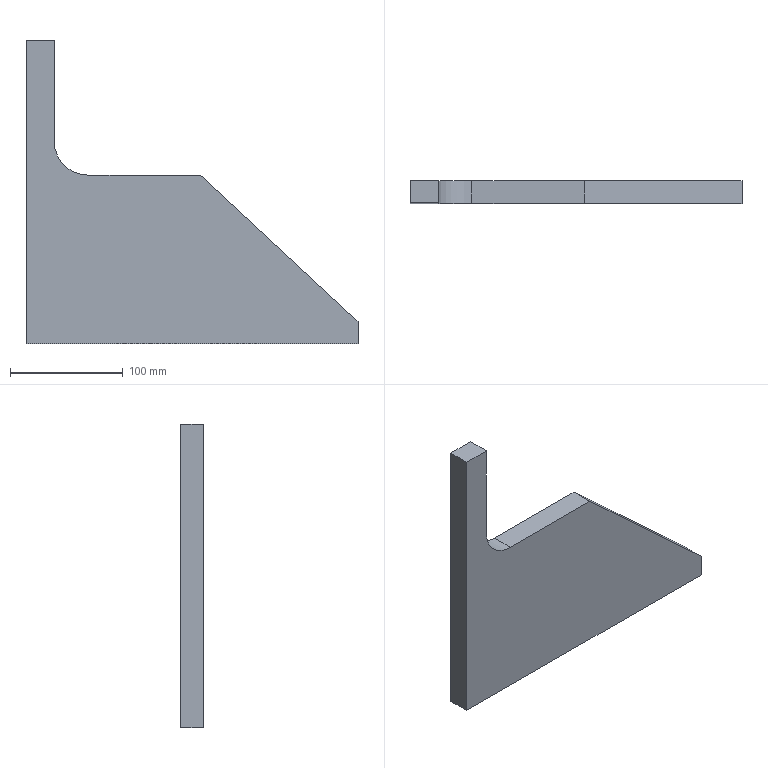Part | STEP file | Tube feed_id778_x_t | 1 solid | 10 faces | box 295 x 20 x 270 mm | volume 766863 mm3 | plane 9 | cylinder 1 | commonest cylinder face diameters 60 x1
STEP:
#1=CARTESIAN_POINT('',(0.,0.,0.));
#2=DIRECTION('',(0.,0.,1.));
#3=DIRECTION('',(1.,0.,0.));
#4=AXIS2_PLACEMENT_3D('',#1,#2,#3);
#5=CARTESIAN_POINT('',(326.,120.936,71.));
#6=VERTEX_POINT('',#5);
#7=CARTESIAN_POINT('',(326.,120.936,-199.));
#8=VERTEX_POINT('',#7);
#9=CARTESIAN_POINT('',(326.,120.936,71.));
#10=DIRECTION('',(0.,0.,-1.));
#11=VECTOR('',#10,1.);
#12=LINE('',#9,#11);
#13=CARTESIAN_POINT('',(326.,140.936,71.));
#14=DIRECTION('',(-1.,0.,0.));
#15=DIRECTION('',(0.,0.,1.));
#16=AXIS2_PLACEMENT_3D('',#13,#14,#15);
#17=PLANE('',#16);
#18=CARTESIAN_POINT('',(0.,-20.));
#19=DIRECTION('',(-1.,0.));
#20=VECTOR('',#19,1.);
#21=LINE('',#18,#20);
#22=(GEOMETRIC_REPRESENTATION_CONTEXT(2)PARAMETRIC_REPRESENTATION_CONTEXT()REPRESENTATION_CONTEXT('',''));
#23=DEFINITIONAL_REPRESENTATION('',(#21),#22);
#24=PCURVE('',#17,#23);
#25=CARTESIAN_POINT('',(0.,120.936,0.));
#26=DIRECTION('',(0.,-1.,0.));
#27=DIRECTION('',(1.,0.,0.));
#28=AXIS2_PLACEMENT_3D('',#25,#26,#27);
#29=PLANE('',#28);
#30=CARTESIAN_POINT('',(326.,71.));
#31=DIRECTION('',(0.,-1.));
#32=VECTOR('',#31,1.);
#33=LINE('',#30,#32);
#34=(GEOMETRIC_REPRESENTATION_CONTEXT(2)PARAMETRIC_REPRESENTATION_CONTEXT()REPRESENTATION_CONTEXT('',''));
#35=DEFINITIONAL_REPRESENTATION('',(#33),#34);
#36=PCURVE('',#29,#35);
#37=SURFACE_CURVE('',#12,(#24,#36),.PCURVE_S1.);
#38=EDGE_CURVE('',#6,#8,#37,.T.);
#39=ORIENTED_EDGE('',*,*,#38,.F.);
#40=CARTESIAN_POINT('',(326.,140.936,71.));
#41=VERTEX_POINT('',#40);
#42=CARTESIAN_POINT('',(326.,140.936,71.));
#43=DIRECTION('',(0.,-1.,0.));
#44=VECTOR('',#43,1.);
#45=LINE('',#42,#44);
#46=CARTESIAN_POINT('',(0.,0.));
#47=DIRECTION('',(0.,-1.));
#48=VECTOR('',#47,1.);
#49=LINE('',#46,#48);
#50=(GEOMETRIC_REPRESENTATION_CONTEXT(2)PARAMETRIC_REPRESENTATION_CONTEXT()REPRESENTATION_CONTEXT('',''));
#51=DEFINITIONAL_REPRESENTATION('',(#49),#50);
#52=PCURVE('',#17,#51);
#53=CARTESIAN_POINT('',(351.,140.936,71.));
#54=DIRECTION('',(0.,0.,1.));
#55=DIRECTION('',(1.,0.,0.));
#56=AXIS2_PLACEMENT_3D('',#53,#54,#55);
#57=PLANE('',#56);
#58=CARTESIAN_POINT('',(-25.,0.));
#59=DIRECTION('',(0.,-1.));
#60=VECTOR('',#59,1.);
#61=LINE('',#58,#60);
#62=(GEOMETRIC_REPRESENTATION_CONTEXT(2)PARAMETRIC_REPRESENTATION_CONTEXT()REPRESENTATION_CONTEXT('',''));
#63=DEFINITIONAL_REPRESENTATION('',(#61),#62);
#64=PCURVE('',#57,#63);
#65=SURFACE_CURVE('',#45,(#52,#64),.PCURVE_S1.);
#66=EDGE_CURVE('',#41,#6,#65,.T.);
#67=ORIENTED_EDGE('',*,*,#66,.F.);
#68=CARTESIAN_POINT('',(326.,140.936,-199.));
#69=VERTEX_POINT('',#68);
#70=CARTESIAN_POINT('',(326.,140.936,71.));
#71=DIRECTION('',(0.,0.,-1.));
#72=VECTOR('',#71,1.);
#73=LINE('',#70,#72);
#74=CARTESIAN_POINT('',(0.,0.));
#75=DIRECTION('',(-1.,0.));
#76=VECTOR('',#75,1.);
#77=LINE('',#74,#76);
#78=(GEOMETRIC_REPRESENTATION_CONTEXT(2)PARAMETRIC_REPRESENTATION_CONTEXT()REPRESENTATION_CONTEXT('',''));
#79=DEFINITIONAL_REPRESENTATION('',(#77),#78);
#80=PCURVE('',#17,#79);
#81=CARTESIAN_POINT('',(0.,140.936,0.));
#82=DIRECTION('',(0.,-1.,0.));
#83=DIRECTION('',(1.,0.,0.));
#84=AXIS2_PLACEMENT_3D('',#81,#82,#83);
#85=PLANE('',#84);
#86=CARTESIAN_POINT('',(326.,71.));
#87=DIRECTION('',(0.,-1.));
#88=VECTOR('',#87,1.);
#89=LINE('',#86,#88);
#90=(GEOMETRIC_REPRESENTATION_CONTEXT(2)PARAMETRIC_REPRESENTATION_CONTEXT()REPRESENTATION_CONTEXT('',''));
#91=DEFINITIONAL_REPRESENTATION('',(#89),#90);
#92=PCURVE('',#85,#91);
#93=SURFACE_CURVE('',#73,(#80,#92),.PCURVE_S1.);
#94=EDGE_CURVE('',#41,#69,#93,.T.);
#95=ORIENTED_EDGE('',*,*,#94,.T.);
#96=CARTESIAN_POINT('',(326.,140.936,-199.));
#97=DIRECTION('',(0.,-1.,0.));
#98=VECTOR('',#97,1.);
#99=LINE('',#96,#98);
#100=CARTESIAN_POINT('',(-270.,0.));
#101=DIRECTION('',(0.,-1.));
#102=VECTOR('',#101,1.);
#103=LINE('',#100,#102);
#104=(GEOMETRIC_REPRESENTATION_CONTEXT(2)PARAMETRIC_REPRESENTATION_CONTEXT()REPRESENTATION_CONTEXT('',''));
#105=DEFINITIONAL_REPRESENTATION('',(#103),#104);
#106=PCURVE('',#17,#105);
#107=CARTESIAN_POINT('',(326.,140.936,-199.));
#108=DIRECTION('',(0.,0.,-1.));
#109=DIRECTION('',(-1.,0.,0.));
#110=AXIS2_PLACEMENT_3D('',#107,#108,#109);
#111=PLANE('',#110);
#112=CARTESIAN_POINT('',(0.,0.));
#113=DIRECTION('',(0.,-1.));
#114=VECTOR('',#113,1.);
#115=LINE('',#112,#114);
#116=(GEOMETRIC_REPRESENTATION_CONTEXT(2)PARAMETRIC_REPRESENTATION_CONTEXT()REPRESENTATION_CONTEXT('',''));
#117=DEFINITIONAL_REPRESENTATION('',(#115),#116);
#118=PCURVE('',#111,#117);
#119=SURFACE_CURVE('',#99,(#106,#118),.PCURVE_S1.);
#120=EDGE_CURVE('',#69,#8,#119,.T.);
#121=ORIENTED_EDGE('',*,*,#120,.T.);
#122=EDGE_LOOP('',(#39,#67,#95,#121));
#123=FACE_BOUND('',#122,.T.);
#124=ADVANCED_FACE('',(#123),#17,.T.);
#125=CARTESIAN_POINT('',(621.,120.936,-199.));
#126=VERTEX_POINT('',#125);
#127=CARTESIAN_POINT('',(326.,120.936,-199.));
#128=DIRECTION('',(1.,0.,0.));
#129=VECTOR('',#128,1.);
#130=LINE('',#127,#129);
#131=CARTESIAN_POINT('',(0.,-20.));
#132=DIRECTION('',(-1.,0.));
#133=VECTOR('',#132,1.);
#134=LINE('',#131,#133);
#135=(GEOMETRIC_REPRESENTATION_CONTEXT(2)PARAMETRIC_REPRESENTATION_CONTEXT()REPRESENTATION_CONTEXT('',''));
#136=DEFINITIONAL_REPRESENTATION('',(#134),#135);
#137=PCURVE('',#111,#136);
#138=CARTESIAN_POINT('',(326.,-199.));
#139=DIRECTION('',(1.,0.));
#140=VECTOR('',#139,1.);
#141=LINE('',#138,#140);
#142=(GEOMETRIC_REPRESENTATION_CONTEXT(2)PARAMETRIC_REPRESENTATION_CONTEXT()REPRESENTATION_CONTEXT('',''));
#143=DEFINITIONAL_REPRESENTATION('',(#141),#142);
#144=PCURVE('',#29,#143);
#145=SURFACE_CURVE('',#130,(#137,#144),.PCURVE_S1.);
#146=EDGE_CURVE('',#8,#126,#145,.T.);
#147=ORIENTED_EDGE('',*,*,#146,.F.);
#148=ORIENTED_EDGE('',*,*,#120,.F.);
#149=CARTESIAN_POINT('',(621.,140.936,-199.));
#150=VERTEX_POINT('',#149);
#151=CARTESIAN_POINT('',(326.,140.936,-199.));
#152=DIRECTION('',(1.,0.,0.));
#153=VECTOR('',#152,1.);
#154=LINE('',#151,#153);
#155=CARTESIAN_POINT('',(0.,0.));
#156=DIRECTION('',(-1.,0.));
#157=VECTOR('',#156,1.);
#158=LINE('',#155,#157);
#159=(GEOMETRIC_REPRESENTATION_CONTEXT(2)PARAMETRIC_REPRESENTATION_CONTEXT()REPRESENTATION_CONTEXT('',''));
#160=DEFINITIONAL_REPRESENTATION('',(#158),#159);
#161=PCURVE('',#111,#160);
#162=CARTESIAN_POINT('',(326.,-199.));
#163=DIRECTION('',(1.,0.));
#164=VECTOR('',#163,1.);
#165=LINE('',#162,#164);
#166=(GEOMETRIC_REPRESENTATION_CONTEXT(2)PARAMETRIC_REPRESENTATION_CONTEXT()REPRESENTATION_CONTEXT('',''));
#167=DEFINITIONAL_REPRESENTATION('',(#165),#166);
#168=PCURVE('',#85,#167);
#169=SURFACE_CURVE('',#154,(#161,#168),.PCURVE_S1.);
#170=EDGE_CURVE('',#69,#150,#169,.T.);
#171=ORIENTED_EDGE('',*,*,#170,.T.);
#172=CARTESIAN_POINT('',(621.,140.936,-199.));
#173=DIRECTION('',(0.,-1.,0.));
#174=VECTOR('',#173,1.);
#175=LINE('',#172,#174);
#176=CARTESIAN_POINT('',(-295.,0.));
#177=DIRECTION('',(0.,-1.));
#178=VECTOR('',#177,1.);
#179=LINE('',#176,#178);
#180=(GEOMETRIC_REPRESENTATION_CONTEXT(2)PARAMETRIC_REPRESENTATION_CONTEXT()REPRESENTATION_CONTEXT('',''));
#181=DEFINITIONAL_REPRESENTATION('',(#179),#180);
#182=PCURVE('',#111,#181);
#183=CARTESIAN_POINT('',(621.,140.936,-199.));
#184=DIRECTION('',(1.,0.,0.));
#185=DIRECTION('',(0.,0.,-1.));
#186=AXIS2_PLACEMENT_3D('',#183,#184,#185);
#187=PLANE('',#186);
#188=CARTESIAN_POINT('',(0.,0.));
#189=DIRECTION('',(0.,-1.));
#190=VECTOR('',#189,1.);
#191=LINE('',#188,#190);
#192=(GEOMETRIC_REPRESENTATION_CONTEXT(2)PARAMETRIC_REPRESENTATION_CONTEXT()REPRESENTATION_CONTEXT('',''));
#193=DEFINITIONAL_REPRESENTATION('',(#191),#192);
#194=PCURVE('',#187,#193);
#195=SURFACE_CURVE('',#175,(#182,#194),.PCURVE_S1.);
#196=EDGE_CURVE('',#150,#126,#195,.T.);
#197=ORIENTED_EDGE('',*,*,#196,.T.);
#198=EDGE_LOOP('',(#147,#148,#171,#197));
#199=FACE_BOUND('',#198,.T.);
#200=ADVANCED_FACE('',(#199),#111,.T.);
#201=CARTESIAN_POINT('',(621.,120.936,-179.));
#202=VERTEX_POINT('',#201);
#203=CARTESIAN_POINT('',(621.,120.936,-199.));
#204=DIRECTION('',(0.,0.,1.));
#205=VECTOR('',#204,1.);
#206=LINE('',#203,#205);
#207=CARTESIAN_POINT('',(0.,-20.));
#208=DIRECTION('',(-1.,0.));
#209=VECTOR('',#208,1.);
#210=LINE('',#207,#209);
#211=(GEOMETRIC_REPRESENTATION_CONTEXT(2)PARAMETRIC_REPRESENTATION_CONTEXT()REPRESENTATION_CONTEXT('',''));
#212=DEFINITIONAL_REPRESENTATION('',(#210),#211);
#213=PCURVE('',#187,#212);
#214=CARTESIAN_POINT('',(621.,-199.));
#215=DIRECTION('',(0.,1.));
#216=VECTOR('',#215,1.);
#217=LINE('',#214,#216);
#218=(GEOMETRIC_REPRESENTATION_CONTEXT(2)PARAMETRIC_REPRESENTATION_CONTEXT()REPRESENTATION_CONTEXT('',''));
#219=DEFINITIONAL_REPRESENTATION('',(#217),#218);
#220=PCURVE('',#29,#219);
#221=SURFACE_CURVE('',#206,(#213,#220),.PCURVE_S1.);
#222=EDGE_CURVE('',#126,#202,#221,.T.);
#223=ORIENTED_EDGE('',*,*,#222,.F.);
#224=ORIENTED_EDGE('',*,*,#196,.F.);
#225=CARTESIAN_POINT('',(621.,140.936,-179.));
#226=VERTEX_POINT('',#225);
#227=CARTESIAN_POINT('',(621.,140.936,-199.));
#228=DIRECTION('',(0.,0.,1.));
#229=VECTOR('',#228,1.);
#230=LINE('',#227,#229);
#231=CARTESIAN_POINT('',(0.,0.));
#232=DIRECTION('',(-1.,0.));
#233=VECTOR('',#232,1.);
#234=LINE('',#231,#233);
#235=(GEOMETRIC_REPRESENTATION_CONTEXT(2)PARAMETRIC_REPRESENTATION_CONTEXT()REPRESENTATION_CONTEXT('',''));
#236=DEFINITIONAL_REPRESENTATION('',(#234),#235);
#237=PCURVE('',#187,#236);
#238=CARTESIAN_POINT('',(621.,-199.));
#239=DIRECTION('',(0.,1.));
#240=VECTOR('',#239,1.);
#241=LINE('',#238,#240);
#242=(GEOMETRIC_REPRESENTATION_CONTEXT(2)PARAMETRIC_REPRESENTATION_CONTEXT()REPRESENTATION_CONTEXT('',''));
#243=DEFINITIONAL_REPRESENTATION('',(#241),#242);
#244=PCURVE('',#85,#243);
#245=SURFACE_CURVE('',#230,(#237,#244),.PCURVE_S1.);
#246=EDGE_CURVE('',#150,#226,#245,.T.);
#247=ORIENTED_EDGE('',*,*,#246,.T.);
#248=CARTESIAN_POINT('',(621.,140.936,-179.));
#249=DIRECTION('',(0.,-1.,0.));
#250=VECTOR('',#249,1.);
#251=LINE('',#248,#250);
#252=CARTESIAN_POINT('',(-20.,0.));
#253=DIRECTION('',(0.,-1.));
#254=VECTOR('',#253,1.);
#255=LINE('',#252,#254);
#256=(GEOMETRIC_REPRESENTATION_CONTEXT(2)PARAMETRIC_REPRESENTATION_CONTEXT()REPRESENTATION_CONTEXT('',''));
#257=DEFINITIONAL_REPRESENTATION('',(#255),#256);
#258=PCURVE('',#187,#257);
#259=CARTESIAN_POINT('',(621.,140.936,-179.));
#260=DIRECTION('',(0.6805,0.,0.7328));
#261=DIRECTION('',(0.7328,0.,-0.6805));
#262=AXIS2_PLACEMENT_3D('',#259,#260,#261);
#263=PLANE('',#262);
#264=CARTESIAN_POINT('',(0.,0.));
#265=DIRECTION('',(0.,-1.));
#266=VECTOR('',#265,1.);
#267=LINE('',#264,#266);
#268=(GEOMETRIC_REPRESENTATION_CONTEXT(2)PARAMETRIC_REPRESENTATION_CONTEXT()REPRESENTATION_CONTEXT('',''));
#269=DEFINITIONAL_REPRESENTATION('',(#267),#268);
#270=PCURVE('',#263,#269);
#271=SURFACE_CURVE('',#251,(#258,#270),.PCURVE_S1.);
#272=EDGE_CURVE('',#226,#202,#271,.T.);
#273=ORIENTED_EDGE('',*,*,#272,.T.);
#274=EDGE_LOOP('',(#223,#224,#247,#273));
#275=FACE_BOUND('',#274,.T.);
#276=ADVANCED_FACE('',(#275),#187,.T.);
#277=CARTESIAN_POINT('',(481.,120.936,-49.));
#278=VERTEX_POINT('',#277);
#279=CARTESIAN_POINT('',(621.,120.936,-179.));
#280=DIRECTION('',(-0.7328,0.,0.6805));
#281=VECTOR('',#280,1.);
#282=LINE('',#279,#281);
#283=CARTESIAN_POINT('',(0.,-20.));
#284=DIRECTION('',(-1.,0.));
#285=VECTOR('',#284,1.);
#286=LINE('',#283,#285);
#287=(GEOMETRIC_REPRESENTATION_CONTEXT(2)PARAMETRIC_REPRESENTATION_CONTEXT()REPRESENTATION_CONTEXT('',''));
#288=DEFINITIONAL_REPRESENTATION('',(#286),#287);
#289=PCURVE('',#263,#288);
#290=CARTESIAN_POINT('',(621.,-179.));
#291=DIRECTION('',(-0.7328,0.6805));
#292=VECTOR('',#291,1.);
#293=LINE('',#290,#292);
#294=(GEOMETRIC_REPRESENTATION_CONTEXT(2)PARAMETRIC_REPRESENTATION_CONTEXT()REPRESENTATION_CONTEXT('',''));
#295=DEFINITIONAL_REPRESENTATION('',(#293),#294);
#296=PCURVE('',#29,#295);
#297=SURFACE_CURVE('',#282,(#289,#296),.PCURVE_S1.);
#298=EDGE_CURVE('',#202,#278,#297,.T.);
#299=ORIENTED_EDGE('',*,*,#298,.F.);
#300=ORIENTED_EDGE('',*,*,#272,.F.);
#301=CARTESIAN_POINT('',(481.,140.936,-49.));
#302=VERTEX_POINT('',#301);
#303=CARTESIAN_POINT('',(621.,140.936,-179.));
#304=DIRECTION('',(-0.7328,0.,0.6805));
#305=VECTOR('',#304,1.);
#306=LINE('',#303,#305);
#307=CARTESIAN_POINT('',(0.,0.));
#308=DIRECTION('',(-1.,0.));
#309=VECTOR('',#308,1.);
#310=LINE('',#307,#309);
#311=(GEOMETRIC_REPRESENTATION_CONTEXT(2)PARAMETRIC_REPRESENTATION_CONTEXT()REPRESENTATION_CONTEXT('',''));
#312=DEFINITIONAL_REPRESENTATION('',(#310),#311);
#313=PCURVE('',#263,#312);
#314=CARTESIAN_POINT('',(621.,-179.));
#315=DIRECTION('',(-0.7328,0.6805));
#316=VECTOR('',#315,1.);
#317=LINE('',#314,#316);
#318=(GEOMETRIC_REPRESENTATION_CONTEXT(2)PARAMETRIC_REPRESENTATION_CONTEXT()REPRESENTATION_CONTEXT('',''));
#319=DEFINITIONAL_REPRESENTATION('',(#317),#318);
#320=PCURVE('',#85,#319);
#321=SURFACE_CURVE('',#306,(#313,#320),.PCURVE_S1.);
#322=EDGE_CURVE('',#226,#302,#321,.T.);
#323=ORIENTED_EDGE('',*,*,#322,.T.);
#324=CARTESIAN_POINT('',(481.,140.936,-49.));
#325=DIRECTION('',(0.,-1.,0.));
#326=VECTOR('',#325,1.);
#327=LINE('',#324,#326);
#328=CARTESIAN_POINT('',(-191.05,0.));
#329=DIRECTION('',(0.,-1.));
#330=VECTOR('',#329,1.);
#331=LINE('',#328,#330);
#332=(GEOMETRIC_REPRESENTATION_CONTEXT(2)PARAMETRIC_REPRESENTATION_CONTEXT()REPRESENTATION_CONTEXT('',''));
#333=DEFINITIONAL_REPRESENTATION('',(#331),#332);
#334=PCURVE('',#263,#333);
#335=CARTESIAN_POINT('',(481.,140.936,-49.));
#336=DIRECTION('',(0.,0.,1.));
#337=DIRECTION('',(1.,0.,0.));
#338=AXIS2_PLACEMENT_3D('',#335,#336,#337);
#339=PLANE('',#338);
#340=CARTESIAN_POINT('',(0.,0.));
#341=DIRECTION('',(0.,-1.));
#342=VECTOR('',#341,1.);
#343=LINE('',#340,#342);
#344=(GEOMETRIC_REPRESENTATION_CONTEXT(2)PARAMETRIC_REPRESENTATION_CONTEXT()REPRESENTATION_CONTEXT('',''));
#345=DEFINITIONAL_REPRESENTATION('',(#343),#344);
#346=PCURVE('',#339,#345);
#347=SURFACE_CURVE('',#327,(#334,#346),.PCURVE_S1.);
#348=EDGE_CURVE('',#302,#278,#347,.T.);
#349=ORIENTED_EDGE('',*,*,#348,.T.);
#350=EDGE_LOOP('',(#299,#300,#323,#349));
#351=FACE_BOUND('',#350,.T.);
#352=ADVANCED_FACE('',(#351),#263,.T.);
#353=CARTESIAN_POINT('',(381.,140.936,-49.));
#354=VERTEX_POINT('',#353);
#355=CARTESIAN_POINT('',(481.,140.936,-49.));
#356=DIRECTION('',(-1.,0.,0.));
#357=VECTOR('',#356,1.);
#358=LINE('',#355,#357);
#359=CARTESIAN_POINT('',(0.,0.));
#360=DIRECTION('',(-1.,0.));
#361=VECTOR('',#360,1.);
#362=LINE('',#359,#361);
#363=(GEOMETRIC_REPRESENTATION_CONTEXT(2)PARAMETRIC_REPRESENTATION_CONTEXT()REPRESENTATION_CONTEXT('',''));
#364=DEFINITIONAL_REPRESENTATION('',(#362),#363);
#365=PCURVE('',#339,#364);
#366=CARTESIAN_POINT('',(481.,-49.));
#367=DIRECTION('',(-1.,0.));
#368=VECTOR('',#367,1.);
#369=LINE('',#366,#368);
#370=(GEOMETRIC_REPRESENTATION_CONTEXT(2)PARAMETRIC_REPRESENTATION_CONTEXT()REPRESENTATION_CONTEXT('',''));
#371=DEFINITIONAL_REPRESENTATION('',(#369),#370);
#372=PCURVE('',#85,#371);
#373=SURFACE_CURVE('',#358,(#365,#372),.PCURVE_S1.);
#374=EDGE_CURVE('',#302,#354,#373,.T.);
#375=ORIENTED_EDGE('',*,*,#374,.T.);
#376=CARTESIAN_POINT('',(381.,120.936,-49.));
#377=VERTEX_POINT('',#376);
#378=CARTESIAN_POINT('',(381.,120.936,-49.));
#379=DIRECTION('',(0.,-1.,0.));
#380=VECTOR('',#379,1.);
#381=LINE('',#378,#380);
#382=CARTESIAN_POINT('',(-100.,-20.));
#383=DIRECTION('',(0.,-1.));
#384=VECTOR('',#383,1.);
#385=LINE('',#382,#384);
#386=(GEOMETRIC_REPRESENTATION_CONTEXT(2)PARAMETRIC_REPRESENTATION_CONTEXT()REPRESENTATION_CONTEXT('',''));
#387=DEFINITIONAL_REPRESENTATION('',(#385),#386);
#388=PCURVE('',#339,#387);
#389=CARTESIAN_POINT('',(381.,140.936,-19.));
#390=DIRECTION('',(0.,1.,0.));
#391=DIRECTION('',(0.,0.,1.));
#392=AXIS2_PLACEMENT_3D('',#389,#390,#391);
#393=CYLINDRICAL_SURFACE('',#392,30.);
#394=CARTESIAN_POINT('',(3.142,-20.));
#395=DIRECTION('',(0.,-1.));
#396=VECTOR('',#395,1.);
#397=LINE('',#394,#396);
#398=(GEOMETRIC_REPRESENTATION_CONTEXT(2)PARAMETRIC_REPRESENTATION_CONTEXT()REPRESENTATION_CONTEXT('',''));
#399=DEFINITIONAL_REPRESENTATION('',(#397),#398);
#400=PCURVE('',#393,#399);
#401=SURFACE_CURVE('',#381,(#388,#400),.PCURVE_S1.);
#402=EDGE_CURVE('',#354,#377,#401,.T.);
#403=ORIENTED_EDGE('',*,*,#402,.T.);
#404=CARTESIAN_POINT('',(481.,120.936,-49.));
#405=DIRECTION('',(-1.,0.,0.));
#406=VECTOR('',#405,1.);
#407=LINE('',#404,#406);
#408=CARTESIAN_POINT('',(0.,-20.));
#409=DIRECTION('',(-1.,0.));
#410=VECTOR('',#409,1.);
#411=LINE('',#408,#410);
#412=(GEOMETRIC_REPRESENTATION_CONTEXT(2)PARAMETRIC_REPRESENTATION_CONTEXT()REPRESENTATION_CONTEXT('',''));
#413=DEFINITIONAL_REPRESENTATION('',(#411),#412);
#414=PCURVE('',#339,#413);
#415=CARTESIAN_POINT('',(481.,-49.));
#416=DIRECTION('',(-1.,0.));
#417=VECTOR('',#416,1.);
#418=LINE('',#415,#417);
#419=(GEOMETRIC_REPRESENTATION_CONTEXT(2)PARAMETRIC_REPRESENTATION_CONTEXT()REPRESENTATION_CONTEXT('',''));
#420=DEFINITIONAL_REPRESENTATION('',(#418),#419);
#421=PCURVE('',#29,#420);
#422=SURFACE_CURVE('',#407,(#414,#421),.PCURVE_S1.);
#423=EDGE_CURVE('',#278,#377,#422,.T.);
#424=ORIENTED_EDGE('',*,*,#423,.F.);
#425=ORIENTED_EDGE('',*,*,#348,.F.);
#426=EDGE_LOOP('',(#375,#403,#424,#425));
#427=FACE_BOUND('',#426,.T.);
#428=ADVANCED_FACE('',(#427),#339,.T.);
#429=CARTESIAN_POINT('',(351.,120.936,-19.));
#430=VERTEX_POINT('',#429);
#431=CARTESIAN_POINT('',(351.,120.936,71.));
#432=VERTEX_POINT('',#431);
#433=CARTESIAN_POINT('',(351.,120.936,-49.));
#434=DIRECTION('',(0.,0.,1.));
#435=VECTOR('',#434,1.);
#436=LINE('',#433,#435);
#437=CARTESIAN_POINT('',(351.,140.936,-49.));
#438=DIRECTION('',(1.,0.,0.));
#439=DIRECTION('',(0.,0.,-1.));
#440=AXIS2_PLACEMENT_3D('',#437,#438,#439);
#441=PLANE('',#440);
#442=CARTESIAN_POINT('',(0.,-20.));
#443=DIRECTION('',(-1.,0.));
#444=VECTOR('',#443,1.);
#445=LINE('',#442,#444);
#446=(GEOMETRIC_REPRESENTATION_CONTEXT(2)PARAMETRIC_REPRESENTATION_CONTEXT()REPRESENTATION_CONTEXT('',''));
#447=DEFINITIONAL_REPRESENTATION('',(#445),#446);
#448=PCURVE('',#441,#447);
#449=CARTESIAN_POINT('',(351.,-49.));
#450=DIRECTION('',(0.,1.));
#451=VECTOR('',#450,1.);
#452=LINE('',#449,#451);
#453=(GEOMETRIC_REPRESENTATION_CONTEXT(2)PARAMETRIC_REPRESENTATION_CONTEXT()REPRESENTATION_CONTEXT('',''));
#454=DEFINITIONAL_REPRESENTATION('',(#452),#453);
#455=PCURVE('',#29,#454);
#456=SURFACE_CURVE('',#436,(#448,#455),.PCURVE_S1.);
#457=EDGE_CURVE('',#430,#432,#456,.T.);
#458=ORIENTED_EDGE('',*,*,#457,.F.);
#459=CARTESIAN_POINT('',(351.,140.936,-19.));
#460=VERTEX_POINT('',#459);
#461=CARTESIAN_POINT('',(351.,140.936,-19.));
#462=DIRECTION('',(0.,1.,0.));
#463=VECTOR('',#462,1.);
#464=LINE('',#461,#463);
#465=CARTESIAN_POINT('',(-30.,0.));
#466=DIRECTION('',(0.,1.));
#467=VECTOR('',#466,1.);
#468=LINE('',#465,#467);
#469=(GEOMETRIC_REPRESENTATION_CONTEXT(2)PARAMETRIC_REPRESENTATION_CONTEXT()REPRESENTATION_CONTEXT('',''));
#470=DEFINITIONAL_REPRESENTATION('',(#468),#469);
#471=PCURVE('',#441,#470);
#472=CARTESIAN_POINT('',(4.712,0.));
#473=DIRECTION('',(0.,1.));
#474=VECTOR('',#473,1.);
#475=LINE('',#472,#474);
#476=(GEOMETRIC_REPRESENTATION_CONTEXT(2)PARAMETRIC_REPRESENTATION_CONTEXT()REPRESENTATION_CONTEXT('',''));
#477=DEFINITIONAL_REPRESENTATION('',(#475),#476);
#478=PCURVE('',#393,#477);
#479=SURFACE_CURVE('',#464,(#471,#478),.PCURVE_S1.);
#480=EDGE_CURVE('',#430,#460,#479,.T.);
#481=ORIENTED_EDGE('',*,*,#480,.T.);
#482=CARTESIAN_POINT('',(351.,140.936,71.));
#483=VERTEX_POINT('',#482);
#484=CARTESIAN_POINT('',(351.,140.936,-49.));
#485=DIRECTION('',(0.,0.,1.));
#486=VECTOR('',#485,1.);
#487=LINE('',#484,#486);
#488=CARTESIAN_POINT('',(0.,0.));
#489=DIRECTION('',(-1.,0.));
#490=VECTOR('',#489,1.);
#491=LINE('',#488,#490);
#492=(GEOMETRIC_REPRESENTATION_CONTEXT(2)PARAMETRIC_REPRESENTATION_CONTEXT()REPRESENTATION_CONTEXT('',''));
#493=DEFINITIONAL_REPRESENTATION('',(#491),#492);
#494=PCURVE('',#441,#493);
#495=CARTESIAN_POINT('',(351.,-49.));
#496=DIRECTION('',(0.,1.));
#497=VECTOR('',#496,1.);
#498=LINE('',#495,#497);
#499=(GEOMETRIC_REPRESENTATION_CONTEXT(2)PARAMETRIC_REPRESENTATION_CONTEXT()REPRESENTATION_CONTEXT('',''));
#500=DEFINITIONAL_REPRESENTATION('',(#498),#499);
#501=PCURVE('',#85,#500);
#502=SURFACE_CURVE('',#487,(#494,#501),.PCURVE_S1.);
#503=EDGE_CURVE('',#460,#483,#502,.T.);
#504=ORIENTED_EDGE('',*,*,#503,.T.);
#505=CARTESIAN_POINT('',(351.,140.936,71.));
#506=DIRECTION('',(0.,-1.,0.));
#507=VECTOR('',#506,1.);
#508=LINE('',#505,#507);
#509=CARTESIAN_POINT('',(-120.,0.));
#510=DIRECTION('',(0.,-1.));
#511=VECTOR('',#510,1.);
#512=LINE('',#509,#511);
#513=(GEOMETRIC_REPRESENTATION_CONTEXT(2)PARAMETRIC_REPRESENTATION_CONTEXT()REPRESENTATION_CONTEXT('',''));
#514=DEFINITIONAL_REPRESENTATION('',(#512),#513);
#515=PCURVE('',#441,#514);
#516=CARTESIAN_POINT('',(0.,0.));
#517=DIRECTION('',(0.,-1.));
#518=VECTOR('',#517,1.);
#519=LINE('',#516,#518);
#520=(GEOMETRIC_REPRESENTATION_CONTEXT(2)PARAMETRIC_REPRESENTATION_CONTEXT()REPRESENTATION_CONTEXT('',''));
#521=DEFINITIONAL_REPRESENTATION('',(#519),#520);
#522=PCURVE('',#57,#521);
#523=SURFACE_CURVE('',#508,(#515,#522),.PCURVE_S1.);
#524=EDGE_CURVE('',#483,#432,#523,.T.);
#525=ORIENTED_EDGE('',*,*,#524,.T.);
#526=EDGE_LOOP('',(#458,#481,#504,#525));
#527=FACE_BOUND('',#526,.T.);
#528=ADVANCED_FACE('',(#527),#441,.T.);
#529=CARTESIAN_POINT('',(351.,120.936,71.));
#530=DIRECTION('',(-1.,0.,0.));
#531=VECTOR('',#530,1.);
#532=LINE('',#529,#531);
#533=CARTESIAN_POINT('',(0.,-20.));
#534=DIRECTION('',(-1.,0.));
#535=VECTOR('',#534,1.);
#536=LINE('',#533,#535);
#537=(GEOMETRIC_REPRESENTATION_CONTEXT(2)PARAMETRIC_REPRESENTATION_CONTEXT()REPRESENTATION_CONTEXT('',''));
#538=DEFINITIONAL_REPRESENTATION('',(#536),#537);
#539=PCURVE('',#57,#538);
#540=CARTESIAN_POINT('',(351.,71.));
#541=DIRECTION('',(-1.,0.));
#542=VECTOR('',#541,1.);
#543=LINE('',#540,#542);
#544=(GEOMETRIC_REPRESENTATION_CONTEXT(2)PARAMETRIC_REPRESENTATION_CONTEXT()REPRESENTATION_CONTEXT('',''));
#545=DEFINITIONAL_REPRESENTATION('',(#543),#544);
#546=PCURVE('',#29,#545);
#547=SURFACE_CURVE('',#532,(#539,#546),.PCURVE_S1.);
#548=EDGE_CURVE('',#432,#6,#547,.T.);
#549=ORIENTED_EDGE('',*,*,#548,.F.);
#550=ORIENTED_EDGE('',*,*,#524,.F.);
#551=CARTESIAN_POINT('',(351.,140.936,71.));
#552=DIRECTION('',(-1.,0.,0.));
#553=VECTOR('',#552,1.);
#554=LINE('',#551,#553);
#555=CARTESIAN_POINT('',(0.,0.));
#556=DIRECTION('',(-1.,0.));
#557=VECTOR('',#556,1.);
#558=LINE('',#555,#557);
#559=(GEOMETRIC_REPRESENTATION_CONTEXT(2)PARAMETRIC_REPRESENTATION_CONTEXT()REPRESENTATION_CONTEXT('',''));
#560=DEFINITIONAL_REPRESENTATION('',(#558),#559);
#561=PCURVE('',#57,#560);
#562=CARTESIAN_POINT('',(351.,71.));
#563=DIRECTION('',(-1.,0.));
#564=VECTOR('',#563,1.);
#565=LINE('',#562,#564);
#566=(GEOMETRIC_REPRESENTATION_CONTEXT(2)PARAMETRIC_REPRESENTATION_CONTEXT()REPRESENTATION_CONTEXT('',''));
#567=DEFINITIONAL_REPRESENTATION('',(#565),#566);
#568=PCURVE('',#85,#567);
#569=SURFACE_CURVE('',#554,(#561,#568),.PCURVE_S1.);
#570=EDGE_CURVE('',#483,#41,#569,.T.);
#571=ORIENTED_EDGE('',*,*,#570,.T.);
#572=ORIENTED_EDGE('',*,*,#66,.T.);
#573=EDGE_LOOP('',(#549,#550,#571,#572));
#574=FACE_BOUND('',#573,.T.);
#575=ADVANCED_FACE('',(#574),#57,.T.);
#576=ORIENTED_EDGE('',*,*,#94,.F.);
#577=ORIENTED_EDGE('',*,*,#570,.F.);
#578=ORIENTED_EDGE('',*,*,#503,.F.);
#579=CARTESIAN_POINT('',(381.,140.936,-19.));
#580=DIRECTION('',(0.,-1.,0.));
#581=DIRECTION('',(1.,0.,0.));
#582=AXIS2_PLACEMENT_3D('',#579,#580,#581);
#583=CIRCLE('',#582,30.);
#584=CARTESIAN_POINT('',(381.,-19.));
#585=DIRECTION('',(1.,0.));
#586=AXIS2_PLACEMENT_2D('',#584,#585);
#587=CIRCLE('',#586,30.);
#588=(GEOMETRIC_REPRESENTATION_CONTEXT(2)PARAMETRIC_REPRESENTATION_CONTEXT()REPRESENTATION_CONTEXT('',''));
#589=DEFINITIONAL_REPRESENTATION('',(#587),#588);
#590=PCURVE('',#85,#589);
#591=CARTESIAN_POINT('',(7.854,0.));
#592=DIRECTION('',(-1.,0.));
#593=VECTOR('',#592,1.);
#594=LINE('',#591,#593);
#595=(GEOMETRIC_REPRESENTATION_CONTEXT(2)PARAMETRIC_REPRESENTATION_CONTEXT()REPRESENTATION_CONTEXT('',''));
#596=DEFINITIONAL_REPRESENTATION('',(#594),#595);
#597=PCURVE('',#393,#596);
#598=SURFACE_CURVE('',#583,(#590,#597),.PCURVE_S1.);
#599=EDGE_CURVE('',#460,#354,#598,.T.);
#600=ORIENTED_EDGE('',*,*,#599,.T.);
#601=ORIENTED_EDGE('',*,*,#374,.F.);
#602=ORIENTED_EDGE('',*,*,#322,.F.);
#603=ORIENTED_EDGE('',*,*,#246,.F.);
#604=ORIENTED_EDGE('',*,*,#170,.F.);
#605=EDGE_LOOP('',(#576,#577,#578,#600,#601,#602,#603,#604));
#606=FACE_BOUND('',#605,.T.);
#607=ADVANCED_FACE('',(#606),#85,.F.);
#608=ORIENTED_EDGE('',*,*,#38,.T.);
#609=ORIENTED_EDGE('',*,*,#146,.T.);
#610=ORIENTED_EDGE('',*,*,#222,.T.);
#611=ORIENTED_EDGE('',*,*,#298,.T.);
#612=ORIENTED_EDGE('',*,*,#423,.T.);
#613=CARTESIAN_POINT('',(381.,120.936,-19.));
#614=DIRECTION('',(0.,1.,0.));
#615=DIRECTION('',(1.,0.,0.));
#616=AXIS2_PLACEMENT_3D('',#613,#614,#615);
#617=CIRCLE('',#616,30.);
#618=CARTESIAN_POINT('',(411.,-19.));
#619=CARTESIAN_POINT('',(411.,-70.962));
#620=CARTESIAN_POINT('',(366.,-44.981));
#621=CARTESIAN_POINT('',(321.,-19.));
#622=CARTESIAN_POINT('',(366.,6.981));
#623=CARTESIAN_POINT('',(411.,32.962));
#624=CARTESIAN_POINT('',(411.,-19.));
#625=(BOUNDED_CURVE()B_SPLINE_CURVE(2,(#618,#619,#620,#621,#622,#623,#624),.UNSPECIFIED.,.T.,.F.)B_SPLINE_CURVE_WITH_KNOTS((1,2,2,2,2,1),(-2.094,0.,2.094,4.189,6.283,8.378),.UNSPECIFIED.)CURVE()GEOMETRIC_REPRESENTATION_ITEM()RATIONAL_B_SPLINE_CURVE((1.,0.5,1.,0.5,1.,0.5,1.))REPRESENTATION_ITEM(''));
#626=(GEOMETRIC_REPRESENTATION_CONTEXT(2)PARAMETRIC_REPRESENTATION_CONTEXT()REPRESENTATION_CONTEXT('',''));
#627=DEFINITIONAL_REPRESENTATION('',(#625),#626);
#628=PCURVE('',#29,#627);
#629=CARTESIAN_POINT('',(1.571,-20.));
#630=DIRECTION('',(1.,0.));
#631=VECTOR('',#630,1.);
#632=LINE('',#629,#631);
#633=(GEOMETRIC_REPRESENTATION_CONTEXT(2)PARAMETRIC_REPRESENTATION_CONTEXT()REPRESENTATION_CONTEXT('',''));
#634=DEFINITIONAL_REPRESENTATION('',(#632),#633);
#635=PCURVE('',#393,#634);
#636=SURFACE_CURVE('',#617,(#628,#635),.PCURVE_S1.);
#637=EDGE_CURVE('',#377,#430,#636,.T.);
#638=ORIENTED_EDGE('',*,*,#637,.T.);
#639=ORIENTED_EDGE('',*,*,#457,.T.);
#640=ORIENTED_EDGE('',*,*,#548,.T.);
#641=EDGE_LOOP('',(#608,#609,#610,#611,#612,#638,#639,#640));
#642=FACE_BOUND('',#641,.T.);
#643=ADVANCED_FACE('',(#642),#29,.T.);
#644=ORIENTED_EDGE('',*,*,#402,.T.);
#645=ORIENTED_EDGE('',*,*,#637,.T.);
#646=ORIENTED_EDGE('',*,*,#480,.T.);
#647=ORIENTED_EDGE('',*,*,#599,.T.);
#648=EDGE_LOOP('',(#644,#645,#646,#647));
#649=FACE_BOUND('',#648,.F.);
#650=ADVANCED_FACE('',(#649),#393,.F.);
#651=CLOSED_SHELL('',(#124,#200,#276,#352,#428,#528,#575,#607,#643,#650));
#652=MANIFOLD_SOLID_BREP('',#651);
#653=(LENGTH_UNIT()NAMED_UNIT(*)SI_UNIT(.MILLI.,.METRE.));
#654=UNCERTAINTY_MEASURE_WITH_UNIT(LENGTH_MEASURE(0.0000001),#653,'','');
#655=(NAMED_UNIT(*)PLANE_ANGLE_UNIT()SI_UNIT($,.RADIAN.));
#656=(NAMED_UNIT(*)SI_UNIT($,.STERADIAN.)SOLID_ANGLE_UNIT());
#657=(GEOMETRIC_REPRESENTATION_CONTEXT(3)GLOBAL_UNCERTAINTY_ASSIGNED_CONTEXT((#654))GLOBAL_UNIT_ASSIGNED_CONTEXT((#653,#655,#656))REPRESENTATION_CONTEXT('',''));
#658=ADVANCED_BREP_SHAPE_REPRESENTATION('',(#4,#652),#657);